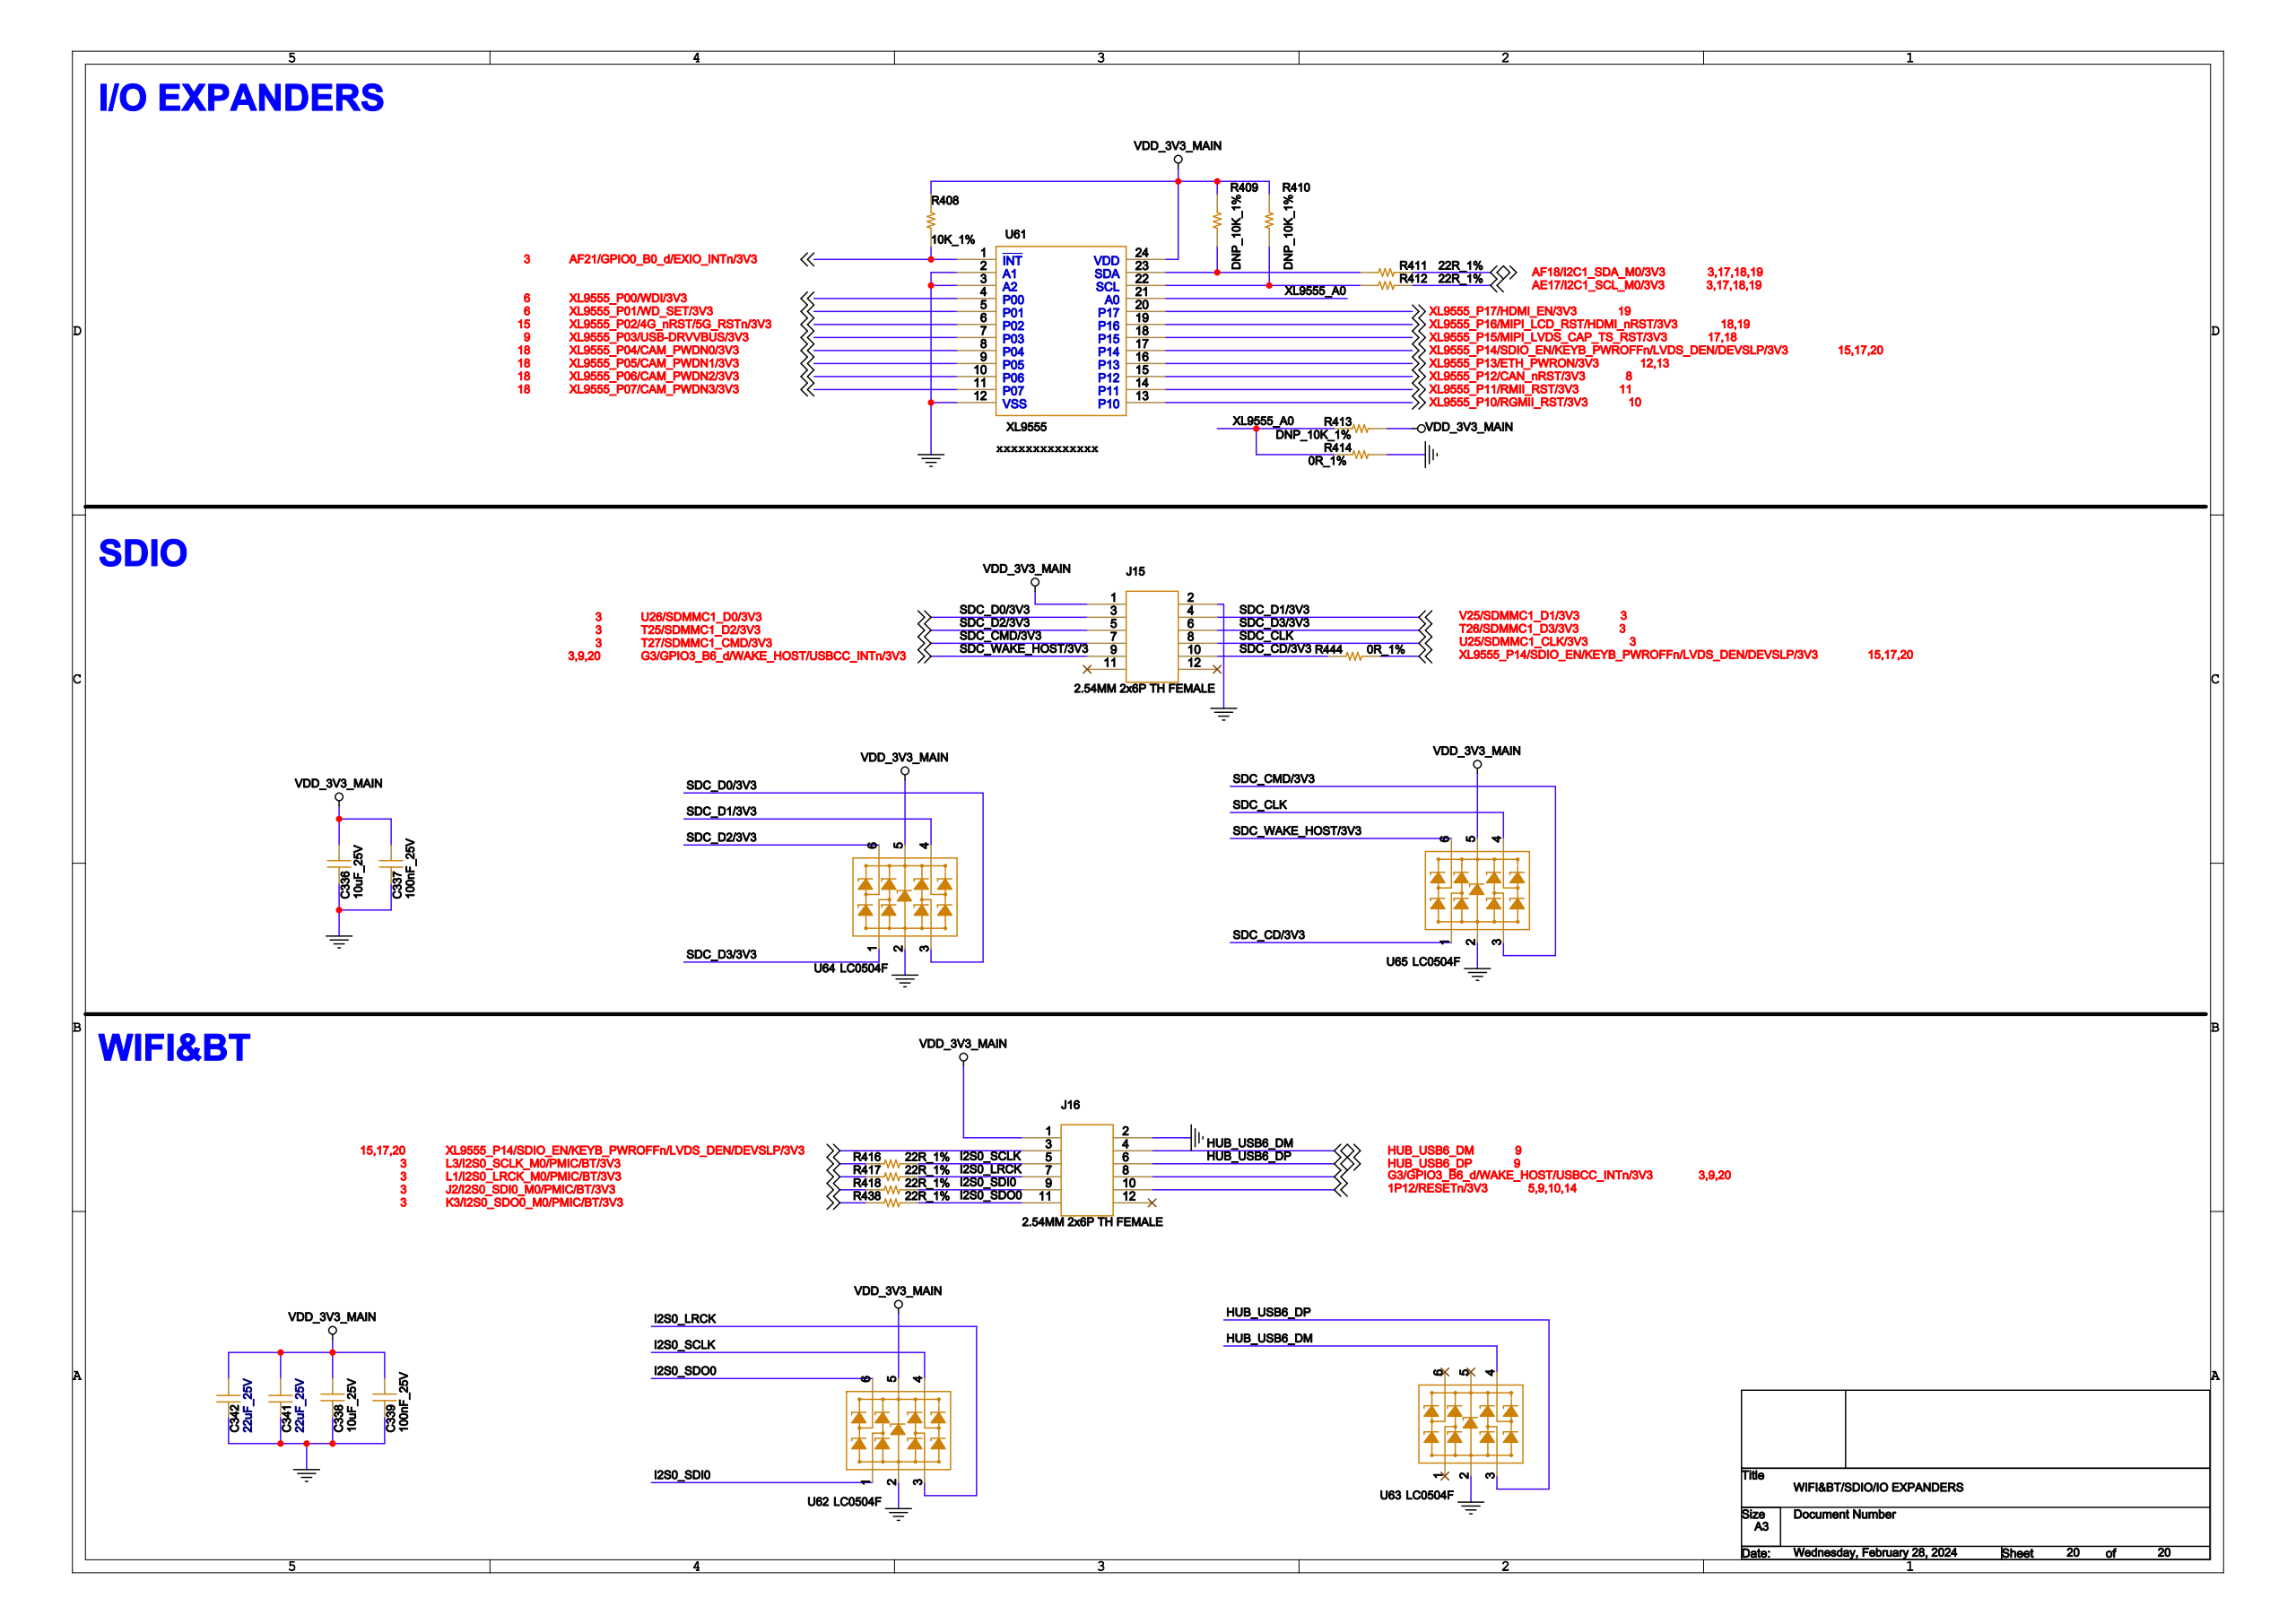Circuit board | Cadence Allegro | 1024 parts | 682 nets | one sheet of the schematic
Parts on this sheet (reference | value | footprint):
C336 | 10uF_25V | C0603
C337 | 100nF_25V | C0402
C338 | 10uF_25V | C0603
C339 | 100nF_25V | C0402
C341 | 22uF_25V | C0805
C342 | 22uF_25V | C0805
J15 | 2.54MM 2x6P TH FEMALE | HEADER_2X6_2D54_MALE
J16 | 2.54MM 2x6P TH FEMALE | HEADER_2X6_2D54_MALE
R408 | 10K_1% | R0402
R409 | DNP_10K_1% | R0402
R410 | DNP_10K_1% | R0402
R411 | 22R_1% | R0402
R412 | 22R_1% | R0402
R413 | DNP_10K_1% | R0402
R414 | 0R_1% | R0603
R416 | 22R_1% | R0402
R417 | 22R_1% | R0402
R418 | 22R_1% | R0402
R438 | 22R_1% | R0402
R444 | 0R_1% | R0402
U61 | XL9555 | TSSOP24
U62 | LC0504F | SOT363
U63 | LC0504F | SOT363
U64 | LC0504F | SOT363
U65 | LC0504F | SOT363
Nets of these parts (net: part-pin ...):
GND: C336-2 C337-2 C338-2 C339-2 C341-1 C342-1 J15-2 J16-2 R414-2 U62-2 U63-2 U64-2 U65-2 U61-2 U61-3 U61-12
VDD_3V3_MAIN: C336-1 C337-1 C338-1 C339-1 C341-2 C342-2 J15-1 J16-1 R408-1 R409-1 R410-1 R413-1 U62-5 U64-5 U65-5 U61-24
1P12/RESETN/3V3: J16-10
AF18/I2C1_SDA_M0/3V3: R411-1
AE17/I2C1_SCL_M0/3V3: R412-1
G3/GPIO3_B6_D/WAKE_HOST/USBCC_I: J15-9 J16-8 U65-6
AF21/GPIO0_B0_D/EXIO_INTN/3V3: R408-2 U61-1
L3/I2S0_SCLK_M0/PMIC/BT/3V3: R416-1
L1/I2S0_LRCK_M0/PMIC/BT/3V3: R417-1
K3/I2S0_SDO0_M0/PMIC/BT/3V3: R438-1
J2/I2S0_SDI0_M0/PMIC/BT/3V3: R418-1
U26/SDMMC1_D0/3V3: J15-3 U64-3
V25/SDMMC1_D1/3V3: J15-4 U64-4
T25/SDMMC1_D2/3V3: J15-5 U64-6
T26/SDMMC1_D3/3V3: J15-6 U64-1
T27/SDMMC1_CMD/3V3: J15-7 U65-3
XL9555_P17/HDMI_EN/3V3: U61-20
XL9555_P03/USB-DRVVBUS/3V3: U61-7
XL9555_A0: R413-2 R414-1 U61-21
XL9555_P11/RMII_RST/3V3: U61-14
XL9555_P00/WDI/3V3: U61-4
XL9555_P01/WD_SET/3V3: U61-5
XL9555_P04/CAM_PWDN0/3V3: U61-8
XL9555_P05/CAM_PWDN1/3V3: U61-9
XL9555_P06/CAM_PWDN2/3V3: U61-10
XL9555_P07/CAM_PWDN3/3V3: U61-11
XL9555_P10/RGMII_RST/3V3: U61-13
XL9555_P13/ETH_PWRON/3V3: U61-16
XL9555_P14/SDIO_EN/KEYB_PWROFFN: J16-3 R444-1 U61-17
N21812872: R410-2 R412-2 U61-22
N21812970: R409-2 R411-2 U61-23
I2S0_SCLK: J16-5 R416-2 U62-4
I2S0_LRCK: J16-7 R417-2 U62-3
I2S0_SDI0: J16-9 R418-2 U62-1
I2S0_SDO0: J16-11 R438-2 U62-6
U25/SDMMC1_CLK/3V3: J15-8 U65-4
SDC_CD/3V3: J15-10 R444-2 U65-1
HUB_USB6_DM: J16-4 U63-4
HUB_USB6_DP: J16-6 U63-3